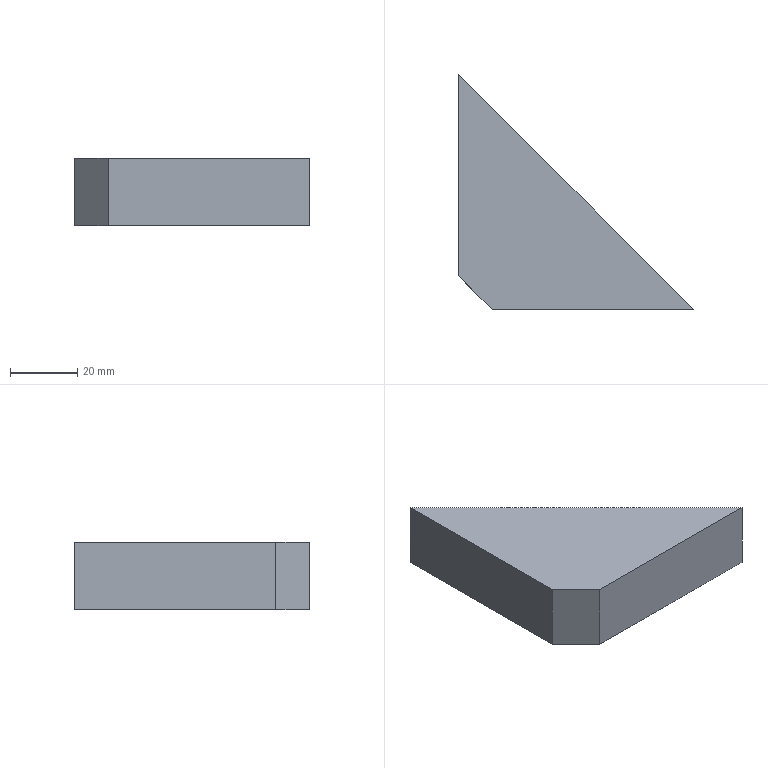Part | SolidWorks | features Chamfer 1, Extrusion 1 | 1 solid | 6 faces | box 70 x 70 x 20 mm | volume 48000 mm3 | plane 6
STEP:
#1=CARTESIAN_POINT('',(70.,0.,0.));
#2=VERTEX_POINT('',#1);
#3=CARTESIAN_POINT('',(0.,70.,0.));
#4=VERTEX_POINT('',#3);
#5=CARTESIAN_POINT('',(70.,0.,0.));
#6=DIRECTION('',(-0.7071,0.7071,0.));
#7=VECTOR('',#6,1000.);
#8=LINE('',#5,#7);
#9=EDGE_CURVE('',#2,#4,#8,.T.);
#10=ORIENTED_EDGE('',*,*,#9,.T.);
#11=CARTESIAN_POINT('',(0.,70.,20.));
#12=VERTEX_POINT('',#11);
#13=CARTESIAN_POINT('',(0.,70.,20.));
#14=DIRECTION('',(0.,0.,-1.));
#15=VECTOR('',#14,1000.);
#16=LINE('',#13,#15);
#17=EDGE_CURVE('',#12,#4,#16,.T.);
#18=ORIENTED_EDGE('',*,*,#17,.F.);
#19=CARTESIAN_POINT('',(70.,0.,20.));
#20=VERTEX_POINT('',#19);
#21=CARTESIAN_POINT('',(70.,0.,20.));
#22=DIRECTION('',(-0.7071,0.7071,0.));
#23=VECTOR('',#22,1000.);
#24=LINE('',#21,#23);
#25=EDGE_CURVE('',#20,#12,#24,.T.);
#26=ORIENTED_EDGE('',*,*,#25,.F.);
#27=CARTESIAN_POINT('',(70.,0.,20.));
#28=DIRECTION('',(0.,0.,-1.));
#29=VECTOR('',#28,1000.);
#30=LINE('',#27,#29);
#31=EDGE_CURVE('',#20,#2,#30,.T.);
#32=ORIENTED_EDGE('',*,*,#31,.T.);
#33=EDGE_LOOP('',(#10,#18,#26,#32));
#34=FACE_OUTER_BOUND('',#33,.T.);
#35=CARTESIAN_POINT('',(70.,0.,20.));
#36=DIRECTION('',(-0.7071,-0.7071,0.));
#37=DIRECTION('',(0.7071,-0.7071,0.));
#38=AXIS2_PLACEMENT_3D('',#35,#36,#37);
#39=PLANE('',#38);
#40=ADVANCED_FACE('',(#34),#39,.F.);
#41=CARTESIAN_POINT('',(0.,10.,0.));
#42=VERTEX_POINT('',#41);
#43=CARTESIAN_POINT('',(0.,70.,0.));
#44=DIRECTION('',(0.,-1.,0.));
#45=VECTOR('',#44,1000.);
#46=LINE('',#43,#45);
#47=EDGE_CURVE('',#4,#42,#46,.T.);
#48=ORIENTED_EDGE('',*,*,#47,.T.);
#49=CARTESIAN_POINT('',(0.,10.,20.));
#50=VERTEX_POINT('',#49);
#51=CARTESIAN_POINT('',(0.,10.,20.));
#52=DIRECTION('',(0.,0.,1.));
#53=VECTOR('',#52,1000.);
#54=LINE('',#51,#53);
#55=EDGE_CURVE('',#42,#50,#54,.T.);
#56=ORIENTED_EDGE('',*,*,#55,.T.);
#57=CARTESIAN_POINT('',(0.,70.,20.));
#58=DIRECTION('',(0.,-1.,0.));
#59=VECTOR('',#58,1000.);
#60=LINE('',#57,#59);
#61=EDGE_CURVE('',#12,#50,#60,.T.);
#62=ORIENTED_EDGE('',*,*,#61,.F.);
#63=ORIENTED_EDGE('',*,*,#17,.T.);
#64=EDGE_LOOP('',(#48,#56,#62,#63));
#65=FACE_OUTER_BOUND('',#64,.T.);
#66=CARTESIAN_POINT('',(0.,70.,20.));
#67=DIRECTION('',(1.,0.,0.));
#68=DIRECTION('',(0.,1.,0.));
#69=AXIS2_PLACEMENT_3D('',#66,#67,#68);
#70=PLANE('',#69);
#71=ADVANCED_FACE('',(#65),#70,.F.);
#72=CARTESIAN_POINT('',(10.,0.,20.));
#73=VERTEX_POINT('',#72);
#74=CARTESIAN_POINT('',(0.,0.,20.));
#75=DIRECTION('',(1.,0.,0.));
#76=VECTOR('',#75,1000.);
#77=LINE('',#74,#76);
#78=EDGE_CURVE('',#73,#20,#77,.T.);
#79=ORIENTED_EDGE('',*,*,#78,.F.);
#80=CARTESIAN_POINT('',(10.,0.,0.));
#81=VERTEX_POINT('',#80);
#82=CARTESIAN_POINT('',(10.,0.,20.));
#83=DIRECTION('',(0.,0.,-1.));
#84=VECTOR('',#83,1000.);
#85=LINE('',#82,#84);
#86=EDGE_CURVE('',#73,#81,#85,.T.);
#87=ORIENTED_EDGE('',*,*,#86,.T.);
#88=CARTESIAN_POINT('',(0.,0.,0.));
#89=DIRECTION('',(1.,0.,0.));
#90=VECTOR('',#89,1000.);
#91=LINE('',#88,#90);
#92=EDGE_CURVE('',#81,#2,#91,.T.);
#93=ORIENTED_EDGE('',*,*,#92,.T.);
#94=ORIENTED_EDGE('',*,*,#31,.F.);
#95=EDGE_LOOP('',(#79,#87,#93,#94));
#96=FACE_OUTER_BOUND('',#95,.T.);
#97=CARTESIAN_POINT('',(0.,0.,20.));
#98=DIRECTION('',(0.,1.,0.));
#99=DIRECTION('',(0.,0.,1.));
#100=AXIS2_PLACEMENT_3D('',#97,#98,#99);
#101=PLANE('',#100);
#102=ADVANCED_FACE('',(#96),#101,.F.);
#103=ORIENTED_EDGE('',*,*,#61,.T.);
#104=CARTESIAN_POINT('',(5.,5.,20.));
#105=DIRECTION('',(0.7071,-0.7071,0.));
#106=VECTOR('',#105,1000.);
#107=LINE('',#104,#106);
#108=EDGE_CURVE('',#50,#73,#107,.T.);
#109=ORIENTED_EDGE('',*,*,#108,.T.);
#110=ORIENTED_EDGE('',*,*,#78,.T.);
#111=ORIENTED_EDGE('',*,*,#25,.T.);
#112=EDGE_LOOP('',(#103,#109,#110,#111));
#113=FACE_OUTER_BOUND('',#112,.T.);
#114=CARTESIAN_POINT('',(0.,0.,20.));
#115=DIRECTION('',(0.,0.,1.));
#116=DIRECTION('',(1.,0.,0.));
#117=AXIS2_PLACEMENT_3D('',#114,#115,#116);
#118=PLANE('',#117);
#119=ADVANCED_FACE('',(#113),#118,.T.);
#120=ORIENTED_EDGE('',*,*,#92,.F.);
#121=CARTESIAN_POINT('',(10.,0.,0.));
#122=DIRECTION('',(-0.7071,0.7071,0.));
#123=VECTOR('',#122,1000.);
#124=LINE('',#121,#123);
#125=EDGE_CURVE('',#81,#42,#124,.T.);
#126=ORIENTED_EDGE('',*,*,#125,.T.);
#127=ORIENTED_EDGE('',*,*,#47,.F.);
#128=ORIENTED_EDGE('',*,*,#9,.F.);
#129=EDGE_LOOP('',(#120,#126,#127,#128));
#130=FACE_OUTER_BOUND('',#129,.T.);
#131=CARTESIAN_POINT('',(0.,0.,0.));
#132=DIRECTION('',(0.,0.,1.));
#133=DIRECTION('',(1.,0.,0.));
#134=AXIS2_PLACEMENT_3D('',#131,#132,#133);
#135=PLANE('',#134);
#136=ADVANCED_FACE('',(#130),#135,.F.);
#137=ORIENTED_EDGE('',*,*,#108,.F.);
#138=ORIENTED_EDGE('',*,*,#55,.F.);
#139=ORIENTED_EDGE('',*,*,#125,.F.);
#140=ORIENTED_EDGE('',*,*,#86,.F.);
#141=EDGE_LOOP('',(#137,#138,#139,#140));
#142=FACE_OUTER_BOUND('',#141,.T.);
#143=CARTESIAN_POINT('',(10.,0.,20.));
#144=DIRECTION('',(0.7071,0.7071,0.));
#145=DIRECTION('',(0.,0.,-1.));
#146=AXIS2_PLACEMENT_3D('',#143,#144,#145);
#147=PLANE('',#146);
#148=ADVANCED_FACE('',(#142),#147,.F.);
#149=CLOSED_SHELL('',(#40,#71,#102,#119,#136,#148));
#150=MANIFOLD_SOLID_BREP('',#149);
#151=CARTESIAN_POINT('',(0.,0.,0.));
#152=DIRECTION('',(0.,0.,1.));
#153=DIRECTION('',(1.,0.,0.));
#154=AXIS2_PLACEMENT_3D('',#151,#152,#153);
#155=(LENGTH_UNIT()NAMED_UNIT(*)SI_UNIT(.MILLI.,.METRE.));
#156=UNCERTAINTY_MEASURE_WITH_UNIT(LENGTH_MEASURE(0.00001),#155,'','');
#157=(NAMED_UNIT(*)PLANE_ANGLE_UNIT()SI_UNIT($,.RADIAN.));
#158=(NAMED_UNIT(*)SI_UNIT($,.STERADIAN.)SOLID_ANGLE_UNIT());
#159=(GEOMETRIC_REPRESENTATION_CONTEXT(3)GLOBAL_UNCERTAINTY_ASSIGNED_CONTEXT((#156))GLOBAL_UNIT_ASSIGNED_CONTEXT((#155,#157,#158))REPRESENTATION_CONTEXT('',''));
#160=ADVANCED_BREP_SHAPE_REPRESENTATION('',(#150,#154),#159);